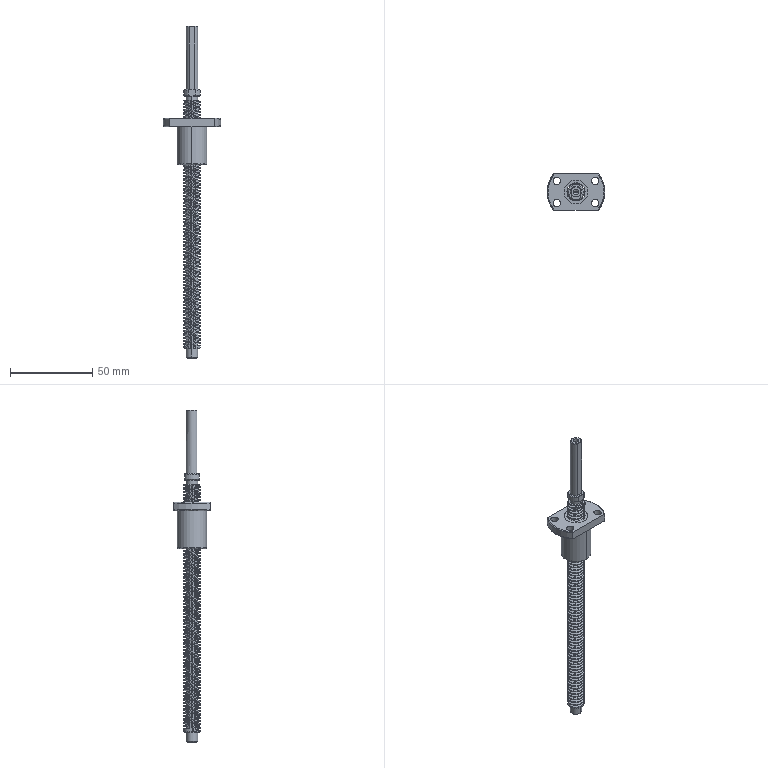Part | NX | features BREP 4 | 4 solids | 235 faces | box 35 x 22 x 201.3 mm | volume 16501 mm3 | cylinder 188 | plane 21 | cone 18 | torus 6 | spline 2 | commonest cylinder face diameters 10 x152 4.5 x8 14.5 x8 11 x6 7 x5 3.3 x4